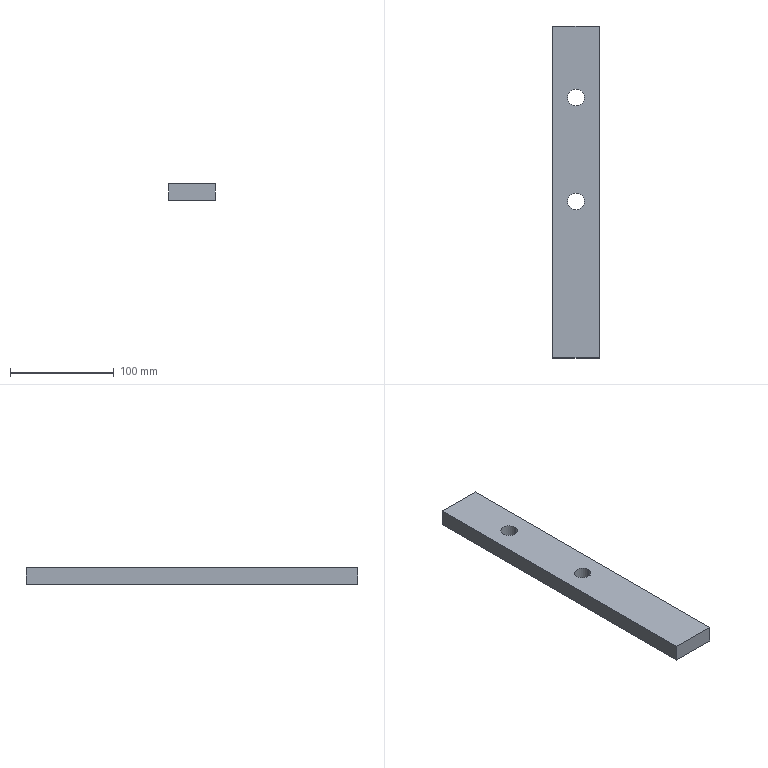Part | SolidWorks | features BaseBody 1 | 1 solid | 10 faces | box 45 x 320 x 16 mm | volume 223966 mm3 | plane 6 | cylinder 4 | commonest cylinder face diameters 16 x4
STEP:
#1=CARTESIAN_POINT('',(14.5,151.,16.));
#2=VERTEX_POINT('',#1);
#3=CARTESIAN_POINT('',(30.5,151.,16.));
#4=VERTEX_POINT('',#3);
#5=CARTESIAN_POINT('',(22.5,151.,16.));
#6=DIRECTION('',(0.,0.,1.));
#7=DIRECTION('',(-1.,0.,0.));
#8=AXIS2_PLACEMENT_3D('',#5,#6,#7);
#9=CIRCLE('',#8,8.);
#10=EDGE_CURVE('',#2,#4,#9,.T.);
#11=ORIENTED_EDGE('',*,*,#10,.T.);
#12=CARTESIAN_POINT('',(30.5,151.,0.));
#13=VERTEX_POINT('',#12);
#14=CARTESIAN_POINT('',(30.5,151.,16.));
#15=DIRECTION('',(0.,0.,-1.));
#16=VECTOR('',#15,1000.);
#17=LINE('',#14,#16);
#18=EDGE_CURVE('',#4,#13,#17,.T.);
#19=ORIENTED_EDGE('',*,*,#18,.T.);
#20=CARTESIAN_POINT('',(14.5,151.,0.));
#21=VERTEX_POINT('',#20);
#22=CARTESIAN_POINT('',(22.5,151.,0.));
#23=DIRECTION('',(0.,0.,1.));
#24=DIRECTION('',(-1.,0.,0.));
#25=AXIS2_PLACEMENT_3D('',#22,#23,#24);
#26=CIRCLE('',#25,8.);
#27=EDGE_CURVE('',#21,#13,#26,.T.);
#28=ORIENTED_EDGE('',*,*,#27,.F.);
#29=CARTESIAN_POINT('',(14.5,151.,16.));
#30=DIRECTION('',(0.,0.,-1.));
#31=VECTOR('',#30,1000.);
#32=LINE('',#29,#31);
#33=EDGE_CURVE('',#2,#21,#32,.T.);
#34=ORIENTED_EDGE('',*,*,#33,.F.);
#35=EDGE_LOOP('',(#11,#19,#28,#34));
#36=FACE_OUTER_BOUND('',#35,.T.);
#37=CARTESIAN_POINT('',(22.5,151.,16.));
#38=DIRECTION('',(0.,0.,-1.));
#39=DIRECTION('',(-1.,0.,0.));
#40=AXIS2_PLACEMENT_3D('',#37,#38,#39);
#41=CYLINDRICAL_SURFACE('',#40,8.);
#42=ADVANCED_FACE('',(#36),#41,.F.);
#43=CARTESIAN_POINT('',(14.5,251.,16.));
#44=VERTEX_POINT('',#43);
#45=CARTESIAN_POINT('',(30.5,251.,16.));
#46=VERTEX_POINT('',#45);
#47=CARTESIAN_POINT('',(22.5,251.,16.));
#48=DIRECTION('',(0.,0.,1.));
#49=DIRECTION('',(-1.,0.,0.));
#50=AXIS2_PLACEMENT_3D('',#47,#48,#49);
#51=CIRCLE('',#50,8.);
#52=EDGE_CURVE('',#44,#46,#51,.T.);
#53=ORIENTED_EDGE('',*,*,#52,.T.);
#54=CARTESIAN_POINT('',(30.5,251.,0.));
#55=VERTEX_POINT('',#54);
#56=CARTESIAN_POINT('',(30.5,251.,16.));
#57=DIRECTION('',(0.,0.,-1.));
#58=VECTOR('',#57,1000.);
#59=LINE('',#56,#58);
#60=EDGE_CURVE('',#46,#55,#59,.T.);
#61=ORIENTED_EDGE('',*,*,#60,.T.);
#62=CARTESIAN_POINT('',(14.5,251.,0.));
#63=VERTEX_POINT('',#62);
#64=CARTESIAN_POINT('',(22.5,251.,0.));
#65=DIRECTION('',(0.,0.,1.));
#66=DIRECTION('',(-1.,0.,0.));
#67=AXIS2_PLACEMENT_3D('',#64,#65,#66);
#68=CIRCLE('',#67,8.);
#69=EDGE_CURVE('',#63,#55,#68,.T.);
#70=ORIENTED_EDGE('',*,*,#69,.F.);
#71=CARTESIAN_POINT('',(14.5,251.,16.));
#72=DIRECTION('',(0.,0.,-1.));
#73=VECTOR('',#72,1000.);
#74=LINE('',#71,#73);
#75=EDGE_CURVE('',#44,#63,#74,.T.);
#76=ORIENTED_EDGE('',*,*,#75,.F.);
#77=EDGE_LOOP('',(#53,#61,#70,#76));
#78=FACE_OUTER_BOUND('',#77,.T.);
#79=CARTESIAN_POINT('',(22.5,251.,16.));
#80=DIRECTION('',(0.,0.,-1.));
#81=DIRECTION('',(-1.,0.,0.));
#82=AXIS2_PLACEMENT_3D('',#79,#80,#81);
#83=CYLINDRICAL_SURFACE('',#82,8.);
#84=ADVANCED_FACE('',(#78),#83,.F.);
#85=CARTESIAN_POINT('',(45.,320.,16.));
#86=VERTEX_POINT('',#85);
#87=CARTESIAN_POINT('',(45.,0.,16.));
#88=VERTEX_POINT('',#87);
#89=CARTESIAN_POINT('',(45.,0.,16.));
#90=DIRECTION('',(0.,-1.,0.));
#91=VECTOR('',#90,1000.);
#92=LINE('',#89,#91);
#93=EDGE_CURVE('',#86,#88,#92,.T.);
#94=ORIENTED_EDGE('',*,*,#93,.F.);
#95=CARTESIAN_POINT('',(0.,320.,16.));
#96=VERTEX_POINT('',#95);
#97=CARTESIAN_POINT('',(0.,320.,16.));
#98=DIRECTION('',(1.,0.,0.));
#99=VECTOR('',#98,1000.);
#100=LINE('',#97,#99);
#101=EDGE_CURVE('',#96,#86,#100,.T.);
#102=ORIENTED_EDGE('',*,*,#101,.F.);
#103=CARTESIAN_POINT('',(0.,0.,16.));
#104=VERTEX_POINT('',#103);
#105=CARTESIAN_POINT('',(0.,0.,16.));
#106=DIRECTION('',(0.,1.,0.));
#107=VECTOR('',#106,1000.);
#108=LINE('',#105,#107);
#109=EDGE_CURVE('',#104,#96,#108,.T.);
#110=ORIENTED_EDGE('',*,*,#109,.F.);
#111=CARTESIAN_POINT('',(0.,0.,16.));
#112=DIRECTION('',(-1.,0.,0.));
#113=VECTOR('',#112,1000.);
#114=LINE('',#111,#113);
#115=EDGE_CURVE('',#88,#104,#114,.T.);
#116=ORIENTED_EDGE('',*,*,#115,.F.);
#117=EDGE_LOOP('',(#94,#102,#110,#116));
#118=FACE_OUTER_BOUND('',#117,.T.);
#119=ORIENTED_EDGE('',*,*,#10,.F.);
#120=CARTESIAN_POINT('',(22.5,151.,16.));
#121=DIRECTION('',(0.,0.,1.));
#122=DIRECTION('',(-1.,0.,0.));
#123=AXIS2_PLACEMENT_3D('',#120,#121,#122);
#124=CIRCLE('',#123,8.);
#125=EDGE_CURVE('',#4,#2,#124,.T.);
#126=ORIENTED_EDGE('',*,*,#125,.F.);
#127=EDGE_LOOP('',(#119,#126));
#128=FACE_BOUND('',#127,.T.);
#129=ORIENTED_EDGE('',*,*,#52,.F.);
#130=CARTESIAN_POINT('',(22.5,251.,16.));
#131=DIRECTION('',(0.,0.,1.));
#132=DIRECTION('',(-1.,0.,0.));
#133=AXIS2_PLACEMENT_3D('',#130,#131,#132);
#134=CIRCLE('',#133,8.);
#135=EDGE_CURVE('',#46,#44,#134,.T.);
#136=ORIENTED_EDGE('',*,*,#135,.F.);
#137=EDGE_LOOP('',(#129,#136));
#138=FACE_BOUND('',#137,.T.);
#139=CARTESIAN_POINT('',(0.,0.,16.));
#140=DIRECTION('',(0.,0.,-1.));
#141=DIRECTION('',(-1.,0.,0.));
#142=AXIS2_PLACEMENT_3D('',#139,#140,#141);
#143=PLANE('',#142);
#144=ADVANCED_FACE('',(#118,#128,#138),#143,.F.);
#145=CARTESIAN_POINT('',(45.,0.,0.));
#146=VERTEX_POINT('',#145);
#147=CARTESIAN_POINT('',(45.,0.,16.));
#148=DIRECTION('',(0.,0.,-1.));
#149=VECTOR('',#148,1000.);
#150=LINE('',#147,#149);
#151=EDGE_CURVE('',#88,#146,#150,.T.);
#152=ORIENTED_EDGE('',*,*,#151,.F.);
#153=ORIENTED_EDGE('',*,*,#115,.T.);
#154=CARTESIAN_POINT('',(0.,0.,0.));
#155=VERTEX_POINT('',#154);
#156=CARTESIAN_POINT('',(0.,0.,16.));
#157=DIRECTION('',(0.,0.,1.));
#158=VECTOR('',#157,1000.);
#159=LINE('',#156,#158);
#160=EDGE_CURVE('',#155,#104,#159,.T.);
#161=ORIENTED_EDGE('',*,*,#160,.F.);
#162=CARTESIAN_POINT('',(45.,0.,0.));
#163=DIRECTION('',(-1.,0.,0.));
#164=VECTOR('',#163,1000.);
#165=LINE('',#162,#164);
#166=EDGE_CURVE('',#146,#155,#165,.T.);
#167=ORIENTED_EDGE('',*,*,#166,.F.);
#168=EDGE_LOOP('',(#152,#153,#161,#167));
#169=FACE_OUTER_BOUND('',#168,.T.);
#170=CARTESIAN_POINT('',(45.,0.,16.));
#171=DIRECTION('',(0.,1.,0.));
#172=DIRECTION('',(-1.,0.,0.));
#173=AXIS2_PLACEMENT_3D('',#170,#171,#172);
#174=PLANE('',#173);
#175=ADVANCED_FACE('',(#169),#174,.F.);
#176=CARTESIAN_POINT('',(45.,320.,0.));
#177=VERTEX_POINT('',#176);
#178=CARTESIAN_POINT('',(45.,320.,16.));
#179=DIRECTION('',(0.,0.,-1.));
#180=VECTOR('',#179,1000.);
#181=LINE('',#178,#180);
#182=EDGE_CURVE('',#86,#177,#181,.T.);
#183=ORIENTED_EDGE('',*,*,#182,.F.);
#184=ORIENTED_EDGE('',*,*,#93,.T.);
#185=ORIENTED_EDGE('',*,*,#151,.T.);
#186=CARTESIAN_POINT('',(45.,320.,0.));
#187=DIRECTION('',(0.,-1.,0.));
#188=VECTOR('',#187,1000.);
#189=LINE('',#186,#188);
#190=EDGE_CURVE('',#177,#146,#189,.T.);
#191=ORIENTED_EDGE('',*,*,#190,.F.);
#192=EDGE_LOOP('',(#183,#184,#185,#191));
#193=FACE_OUTER_BOUND('',#192,.T.);
#194=CARTESIAN_POINT('',(45.,320.,16.));
#195=DIRECTION('',(-1.,0.,0.));
#196=DIRECTION('',(0.,-1.,0.));
#197=AXIS2_PLACEMENT_3D('',#194,#195,#196);
#198=PLANE('',#197);
#199=ADVANCED_FACE('',(#193),#198,.F.);
#200=CARTESIAN_POINT('',(0.,320.,0.));
#201=VERTEX_POINT('',#200);
#202=CARTESIAN_POINT('',(0.,320.,16.));
#203=DIRECTION('',(0.,0.,-1.));
#204=VECTOR('',#203,1000.);
#205=LINE('',#202,#204);
#206=EDGE_CURVE('',#96,#201,#205,.T.);
#207=ORIENTED_EDGE('',*,*,#206,.F.);
#208=ORIENTED_EDGE('',*,*,#101,.T.);
#209=ORIENTED_EDGE('',*,*,#182,.T.);
#210=CARTESIAN_POINT('',(0.,320.,0.));
#211=DIRECTION('',(1.,0.,0.));
#212=VECTOR('',#211,1000.);
#213=LINE('',#210,#212);
#214=EDGE_CURVE('',#201,#177,#213,.T.);
#215=ORIENTED_EDGE('',*,*,#214,.F.);
#216=EDGE_LOOP('',(#207,#208,#209,#215));
#217=FACE_OUTER_BOUND('',#216,.T.);
#218=CARTESIAN_POINT('',(0.,320.,16.));
#219=DIRECTION('',(0.,-1.,0.));
#220=DIRECTION('',(0.,0.,-1.));
#221=AXIS2_PLACEMENT_3D('',#218,#219,#220);
#222=PLANE('',#221);
#223=ADVANCED_FACE('',(#217),#222,.F.);
#224=ORIENTED_EDGE('',*,*,#160,.T.);
#225=ORIENTED_EDGE('',*,*,#109,.T.);
#226=ORIENTED_EDGE('',*,*,#206,.T.);
#227=CARTESIAN_POINT('',(0.,0.,0.));
#228=DIRECTION('',(0.,1.,0.));
#229=VECTOR('',#228,1000.);
#230=LINE('',#227,#229);
#231=EDGE_CURVE('',#155,#201,#230,.T.);
#232=ORIENTED_EDGE('',*,*,#231,.F.);
#233=EDGE_LOOP('',(#224,#225,#226,#232));
#234=FACE_OUTER_BOUND('',#233,.T.);
#235=CARTESIAN_POINT('',(0.,0.,16.));
#236=DIRECTION('',(1.,0.,0.));
#237=DIRECTION('',(0.,0.,-1.));
#238=AXIS2_PLACEMENT_3D('',#235,#236,#237);
#239=PLANE('',#238);
#240=ADVANCED_FACE('',(#234),#239,.F.);
#241=ORIENTED_EDGE('',*,*,#18,.F.);
#242=ORIENTED_EDGE('',*,*,#125,.T.);
#243=ORIENTED_EDGE('',*,*,#33,.T.);
#244=CARTESIAN_POINT('',(22.5,151.,0.));
#245=DIRECTION('',(0.,0.,1.));
#246=DIRECTION('',(-1.,0.,0.));
#247=AXIS2_PLACEMENT_3D('',#244,#245,#246);
#248=CIRCLE('',#247,8.);
#249=EDGE_CURVE('',#13,#21,#248,.T.);
#250=ORIENTED_EDGE('',*,*,#249,.F.);
#251=EDGE_LOOP('',(#241,#242,#243,#250));
#252=FACE_OUTER_BOUND('',#251,.T.);
#253=CARTESIAN_POINT('',(22.5,151.,16.));
#254=DIRECTION('',(0.,0.,-1.));
#255=DIRECTION('',(-1.,0.,0.));
#256=AXIS2_PLACEMENT_3D('',#253,#254,#255);
#257=CYLINDRICAL_SURFACE('',#256,8.);
#258=ADVANCED_FACE('',(#252),#257,.F.);
#259=ORIENTED_EDGE('',*,*,#60,.F.);
#260=ORIENTED_EDGE('',*,*,#135,.T.);
#261=ORIENTED_EDGE('',*,*,#75,.T.);
#262=CARTESIAN_POINT('',(22.5,251.,0.));
#263=DIRECTION('',(0.,0.,1.));
#264=DIRECTION('',(-1.,0.,0.));
#265=AXIS2_PLACEMENT_3D('',#262,#263,#264);
#266=CIRCLE('',#265,8.);
#267=EDGE_CURVE('',#55,#63,#266,.T.);
#268=ORIENTED_EDGE('',*,*,#267,.F.);
#269=EDGE_LOOP('',(#259,#260,#261,#268));
#270=FACE_OUTER_BOUND('',#269,.T.);
#271=CARTESIAN_POINT('',(22.5,251.,16.));
#272=DIRECTION('',(0.,0.,-1.));
#273=DIRECTION('',(-1.,0.,0.));
#274=AXIS2_PLACEMENT_3D('',#271,#272,#273);
#275=CYLINDRICAL_SURFACE('',#274,8.);
#276=ADVANCED_FACE('',(#270),#275,.F.);
#277=ORIENTED_EDGE('',*,*,#214,.T.);
#278=ORIENTED_EDGE('',*,*,#190,.T.);
#279=ORIENTED_EDGE('',*,*,#166,.T.);
#280=ORIENTED_EDGE('',*,*,#231,.T.);
#281=EDGE_LOOP('',(#277,#278,#279,#280));
#282=FACE_OUTER_BOUND('',#281,.T.);
#283=ORIENTED_EDGE('',*,*,#27,.T.);
#284=ORIENTED_EDGE('',*,*,#249,.T.);
#285=EDGE_LOOP('',(#283,#284));
#286=FACE_BOUND('',#285,.T.);
#287=ORIENTED_EDGE('',*,*,#69,.T.);
#288=ORIENTED_EDGE('',*,*,#267,.T.);
#289=EDGE_LOOP('',(#287,#288));
#290=FACE_BOUND('',#289,.T.);
#291=CARTESIAN_POINT('',(0.,0.,0.));
#292=DIRECTION('',(0.,0.,-1.));
#293=DIRECTION('',(-1.,0.,0.));
#294=AXIS2_PLACEMENT_3D('',#291,#292,#293);
#295=PLANE('',#294);
#296=ADVANCED_FACE('',(#282,#286,#290),#295,.T.);
#297=CLOSED_SHELL('',(#42,#84,#144,#175,#199,#223,#240,#258,#276,#296));
#298=MANIFOLD_SOLID_BREP('',#297);
#299=CARTESIAN_POINT('',(0.,0.,0.));
#300=DIRECTION('',(0.,0.,1.));
#301=DIRECTION('',(1.,0.,0.));
#302=AXIS2_PLACEMENT_3D('',#299,#300,#301);
#303=(LENGTH_UNIT()NAMED_UNIT(*)SI_UNIT(.MILLI.,.METRE.));
#304=UNCERTAINTY_MEASURE_WITH_UNIT(LENGTH_MEASURE(0.00001),#303,'','');
#305=(NAMED_UNIT(*)PLANE_ANGLE_UNIT()SI_UNIT($,.RADIAN.));
#306=(NAMED_UNIT(*)SI_UNIT($,.STERADIAN.)SOLID_ANGLE_UNIT());
#307=(GEOMETRIC_REPRESENTATION_CONTEXT(3)GLOBAL_UNCERTAINTY_ASSIGNED_CONTEXT((#304))GLOBAL_UNIT_ASSIGNED_CONTEXT((#303,#305,#306))REPRESENTATION_CONTEXT('',''));
#308=ADVANCED_BREP_SHAPE_REPRESENTATION('',(#298,#302),#307);